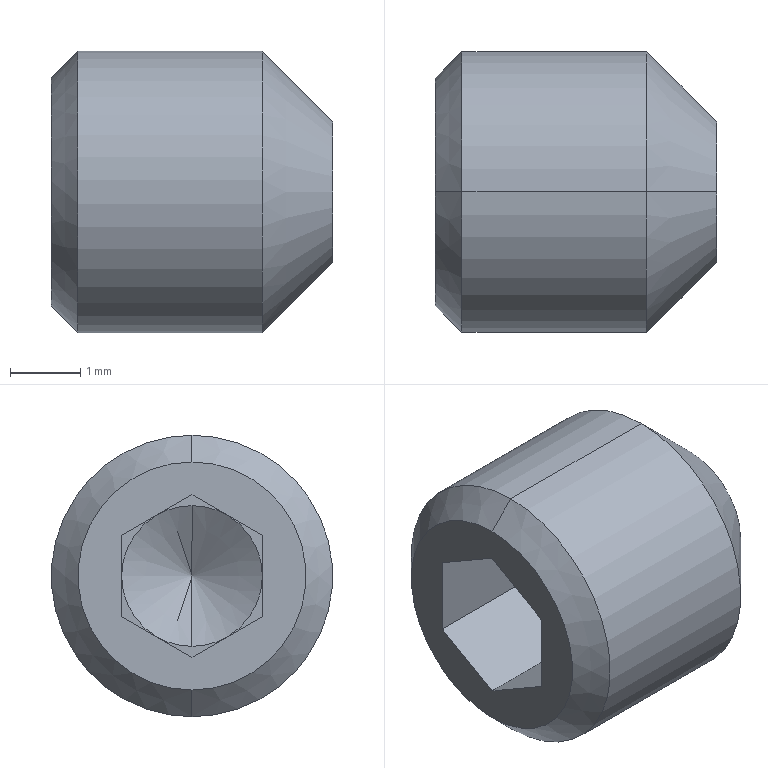Part | STEP file | hexagon socket set screws with cup point gb_GB_SOCKET_SET_TYPE4 M4X4-N.step-24.STEP.STEP-96.STEP | 1 solid | 24 faces | box 4 x 4 x 4 mm | volume 38.012 mm3 | plane 14 | cone 8 | cylinder 2 | commonest cylinder face diameters 4 x2